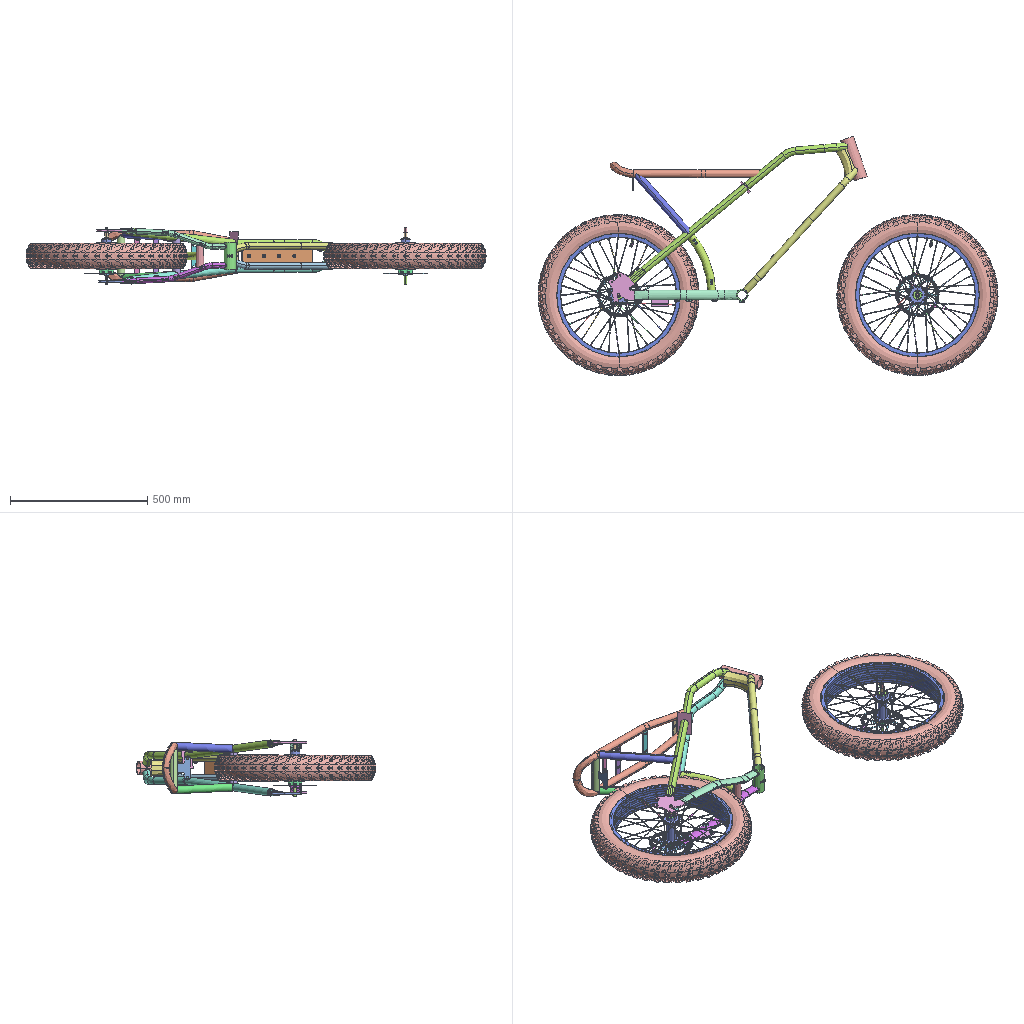Assembly | STEP file | 125 different items | 225 placed | box 1675 x 872 x 210 mm
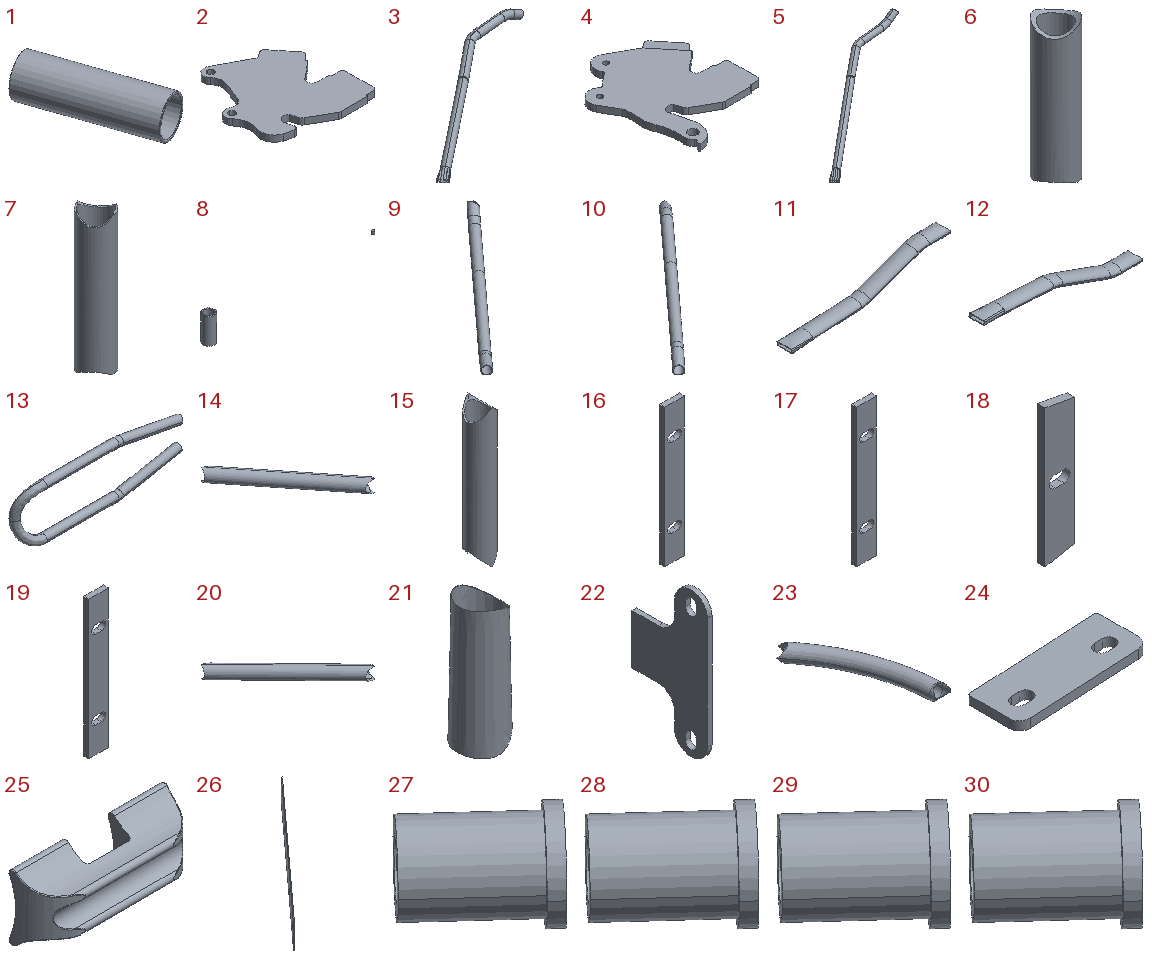Parts list (item | name | quantity | parent item | size | volume):
1 | PRT0001_68_1 | x1 | in PRT0001_68_ASM | 97.464 x 162.507 x 50 mm | 68590 mm3
2 | PRT0001_68_2 | x1 | in PRT0001_68_ASM | 96.462 x 102.711 x 6 mm | 37428 mm3
3 | PRT0001_68_3 | x1 | in PRT0001_68_ASM | 800.156 x 514.114 x 98.789 mm | 118663 mm3
4 | PRT0001_68_4 | x1 | in PRT0001_68_ASM | 102.996 x 124.109 x 6.875 mm | 43677 mm3
5 | PRT0001_68_5 | x1 | in PRT0001_68_ASM | 800.156 x 514.114 x 98.789 mm | 118661 mm3
6 | PRT0001_68_6 | x1 | in PRT0001_68_ASM | 19.001 x 19.001 x 71.436 mm | 7755 mm3
7 | PRT0001_68_7 | x1 | in PRT0001_68_ASM | 28.01 x 28.01 x 125 mm | 14806 mm3
8 | PRT0001_68_8 | x1 | in PRT0001_68_ASM | 664.5 x 43 x 100 mm | 56748 mm3
9 | PRT0001_68_9 | x1 | in PRT0001_68_ASM | 418.507 x 458.308 x 40.27 mm | 65357 mm3
10 | PRT0001_68_10 | x1 | in PRT0001_68_ASM | 418.507 x 458.308 x 40.27 mm | 65357 mm3
11 | PRT0001_68_11 | x1 | in PRT0001_68_ASM | 380.555 x 36.2 x 75.962 mm | 44196 mm3
12 | PRT0001_68_12 | x1 | in PRT0001_68_ASM | 380.555 x 36.2 x 75.962 mm | 44196 mm3
13 | PRT0001_68_13 | x1 | in PRT0001_68_ASM | 553.703 x 55.695 x 188 mm | 147514 mm3
14 | PRT0001_68_15 | x1 | in PRT0001_68_ASM | 199.467 x 218.482 x 38.316 mm | 33314 mm3
15 | PRT0001_68_16 | x1 | in PRT0001_68_ASM | 28 x 28 x 159.999 mm | 17361 mm3
16 | PRT0001_68_17 | x1 | in PRT0001_68_ASM | 20 x 5 x 138.552 mm | 12873 mm3
17 | PRT0001_68_18 | x1 | in PRT0001_68_ASM | 20 x 5 x 138.552 mm | 12873 mm3
18 | PRT0001_68_19 | x1 | in PRT0001_68_ASM | 20 x 5 x 93.385 mm | 8469 mm3
19 | PRT0001_68_20 | x1 | in PRT0001_68_ASM | 20 x 5.003 x 138.552 mm | 12879 mm3
20 | PRT0001_68_21 | x1 | in PRT0001_68_ASM | 199.467 x 218.482 x 38.316 mm | 33312 mm3
21 | PRT0001_68_22 | x1 | in PRT0001_68_ASM | 29.224 x 29.394 x 81.102 mm | 9192 mm3
22 | PRT0001_68_23 | x1 | in PRT0001_68_ASM | 2.865 x 46.012 x 88.1 mm | 6874 mm3
23 | PRT0001_68_24 | x1 | in PRT0001_68_ASM | 109.297 x 231.955 x 28 mm | 28262 mm3
24 | PRT0001_68_25 | x1 | in PRT0001_68_ASM | 62.055 x 25 x 7.544 mm | 6128 mm3
25 | PRT0001_68_27 | x11 | in PRT0001_68_ASM, PRT0001_ASM | 19.974 x 5.821 x 8.525 mm | 410.28 mm3
26 | PRT0001_68_28 | x1 | in PRT0001_68_ASM | 256.776 x 282.202 x 48 mm | 26740 mm3
27 | PRT0001_68_29 | x1 | in PRT0001_68_ASM | 20.651 x 20.315 x 13 mm | 1037 mm3
28 | PRT0001_68_30 | x1 | in PRT0001_68_ASM | 20.651 x 20.315 x 13 mm | 1037 mm3
29 | PRT0001_68_31 | x1 | in PRT0001_68_ASM | 20.651 x 20.315 x 13 mm | 1037 mm3
30 | PRT0001_68_32 | x1 | in PRT0001_68_ASM | 20.651 x 20.315 x 13 mm | 1037 mm3
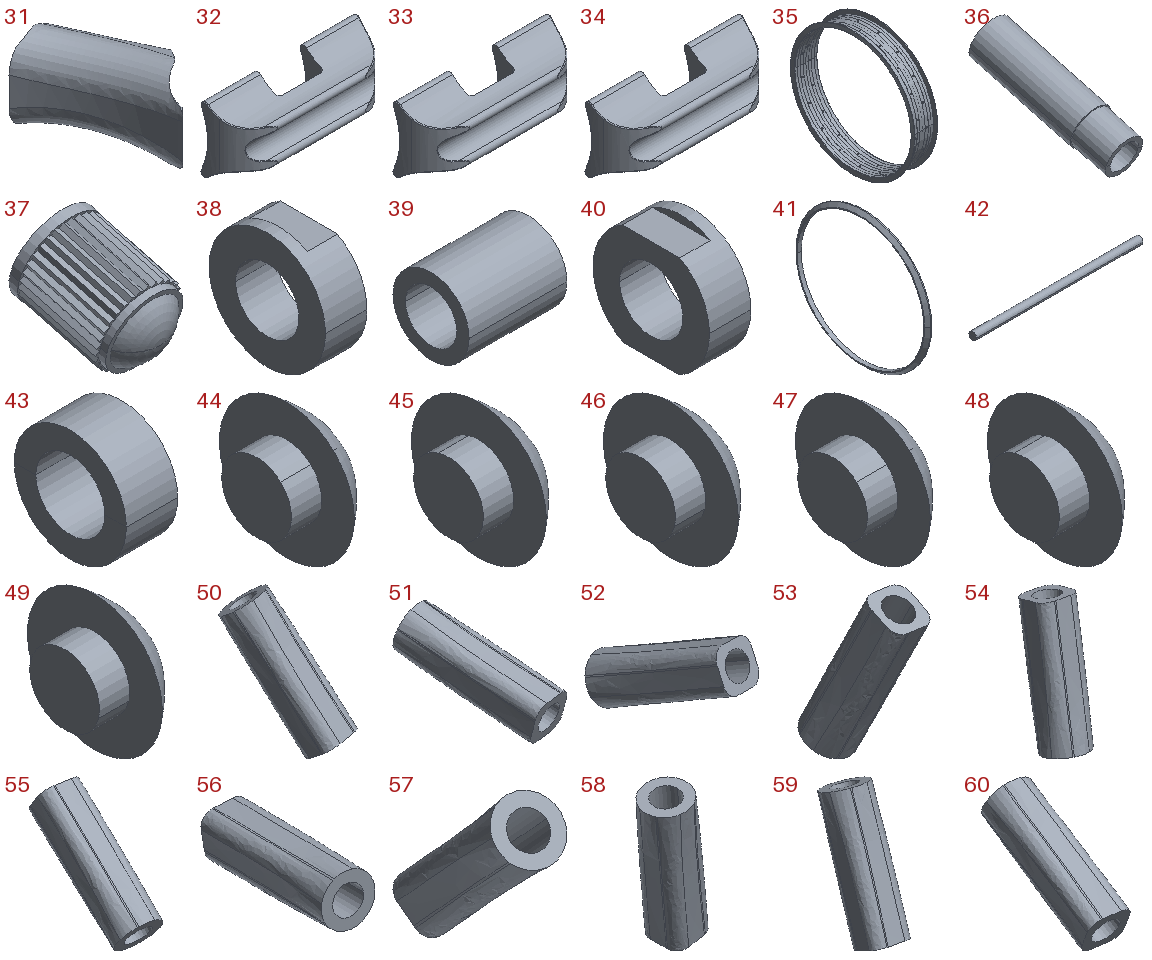31 | PRT0001_68_33 | x1 | in PRT0001_68_ASM | 68.382 x 110.355 x 61.109 mm | 20597 mm3
32 | PRT0003 | x1 | in PRT0001_ASM | 19.974 x 5.821 x 8.525 mm | 410.28 mm3
33 | PRT0004 | x1 | in PRT0001_ASM | 19.974 x 5.821 x 8.525 mm | 410.28 mm3
34 | PRT0005 | x1 | in PRT0001_ASM | 19.974 x 5.821 x 8.525 mm | 410.28 mm3
35 | BREP_1 | x2 | in FATBIKE20X4INCHFRONTWHEELAVID16_ASM | 83.255 x 451.856 x 451.856 mm | 216324 mm3
36 | BREP_2 | x2 | in FATBIKE20X4INCHFRONTWHEELAVID16_ASM | 8 x 29.756 x 14.922 mm | 672.27 mm3
37 | BREP_3 | x2 | in FATBIKE20X4INCHFRONTWHEELAVID16_ASM | 10.16 x 14.692 x 12.577 mm | 395.376 mm3
38 | BREP_4 | x2 | in FATBIKE20X4INCHFRONTWHEELAVID16_ASM | 6.16 x 17.28 x 17.28 mm | 959.564 mm3
39 | BREP_5 | x2 | in FATBIKE20X4INCHFRONTWHEELAVID16_ASM | 18 x 14 x 14 mm | 1522 mm3
40 | BREP_6 | x2 | in FATBIKE20X4INCHFRONTWHEELAVID16_ASM | 6.16 x 17.28 x 17.28 mm | 959.564 mm3
41 | BREP_7 | x2 | in FATBIKE20X4INCHFRONTWHEELAVID16_ASM | 1 x 33.32 x 33.32 mm | 72.205 mm3
42 | BREP_8 | x2 | in FATBIKE20X4INCHFRONTWHEELAVID16_ASM | 210 x 9.4 x 9.4 mm | 14574 mm3
43 | BREP_9 | x2 | in FATBIKE20X4INCHFRONTWHEELAVID16_ASM | 7 x 15.25 x 15.25 mm | 792.795 mm3
44 | OBJECT_38-2315 | x2 | in FATBIKE20X4INCHFRONTWHEELAVID16_ASM | 3.344 x 7.727 x 7.727 mm | 53.316 mm3
45 | OBJECT_38-2316 | x2 | in FATBIKE20X4INCHFRONTWHEELAVID16_ASM | 3.344 x 7.727 x 7.727 mm | 53.316 mm3
46 | OBJECT_38-2317 | x2 | in FATBIKE20X4INCHFRONTWHEELAVID16_ASM | 3.344 x 7.727 x 7.727 mm | 53.316 mm3
47 | OBJECT_38-2318 | x2 | in FATBIKE20X4INCHFRONTWHEELAVID16_ASM | 3.344 x 7.727 x 7.727 mm | 53.316 mm3
48 | OBJECT_38-2319 | x2 | in FATBIKE20X4INCHFRONTWHEELAVID16_ASM | 3.344 x 7.727 x 7.727 mm | 53.316 mm3
49 | OBJECT_38-2320 | x2 | in FATBIKE20X4INCHFRONTWHEELAVID16_ASM | 3.344 x 7.727 x 7.727 mm | 53.316 mm3
50 | BREP_16 | x2 | in FATBIKE20X4INCHFRONTWHEELAVID16_ASM | 5.376 x 10.304 x 11.842 mm | 92.736 mm3
51 | BREP_17 | x2 | in FATBIKE20X4INCHFRONTWHEELAVID16_ASM | 5.376 x 12.643 x 6.336 mm | 92.736 mm3
52 | BREP_18 | x2 | in FATBIKE20X4INCHFRONTWHEELAVID16_ASM | 5.376 x 12.425 x 8.884 mm | 92.736 mm3
53 | BREP_19 | x2 | in FATBIKE20X4INCHFRONTWHEELAVID16_ASM | 5.376 x 8.093 x 12.59 mm | 92.736 mm3
54 | BREP_20 | x2 | in FATBIKE20X4INCHFRONTWHEELAVID16_ASM | 5.376 x 7.197 x 12.647 mm | 92.736 mm3
55 | BREP_21 | x2 | in FATBIKE20X4INCHFRONTWHEELAVID16_ASM | 5.376 x 12.182 x 9.645 mm | 92.736 mm3
56 | BREP_22 | x2 | in FATBIKE20X4INCHFRONTWHEELAVID16_ASM | 5.376 x 12.545 x 5.293 mm | 92.736 mm3
57 | BREP_23 | x2 | in FATBIKE20X4INCHFRONTWHEELAVID16_ASM | 5.376 x 10.907 x 11.414 mm | 92.736 mm3
58 | BREP_24 | x2 | in FATBIKE20X4INCHFRONTWHEELAVID16_ASM | 5.376 x 4.387 x 12.44 mm | 92.736 mm3
59 | BREP_25 | x2 | in FATBIKE20X4INCHFRONTWHEELAVID16_ASM | 5.376 x 8.884 x 12.425 mm | 92.736 mm3
60 | BREP_26 | x2 | in FATBIKE20X4INCHFRONTWHEELAVID16_ASM | 5.376 x 12.59 x 8.093 mm | 92.736 mm3
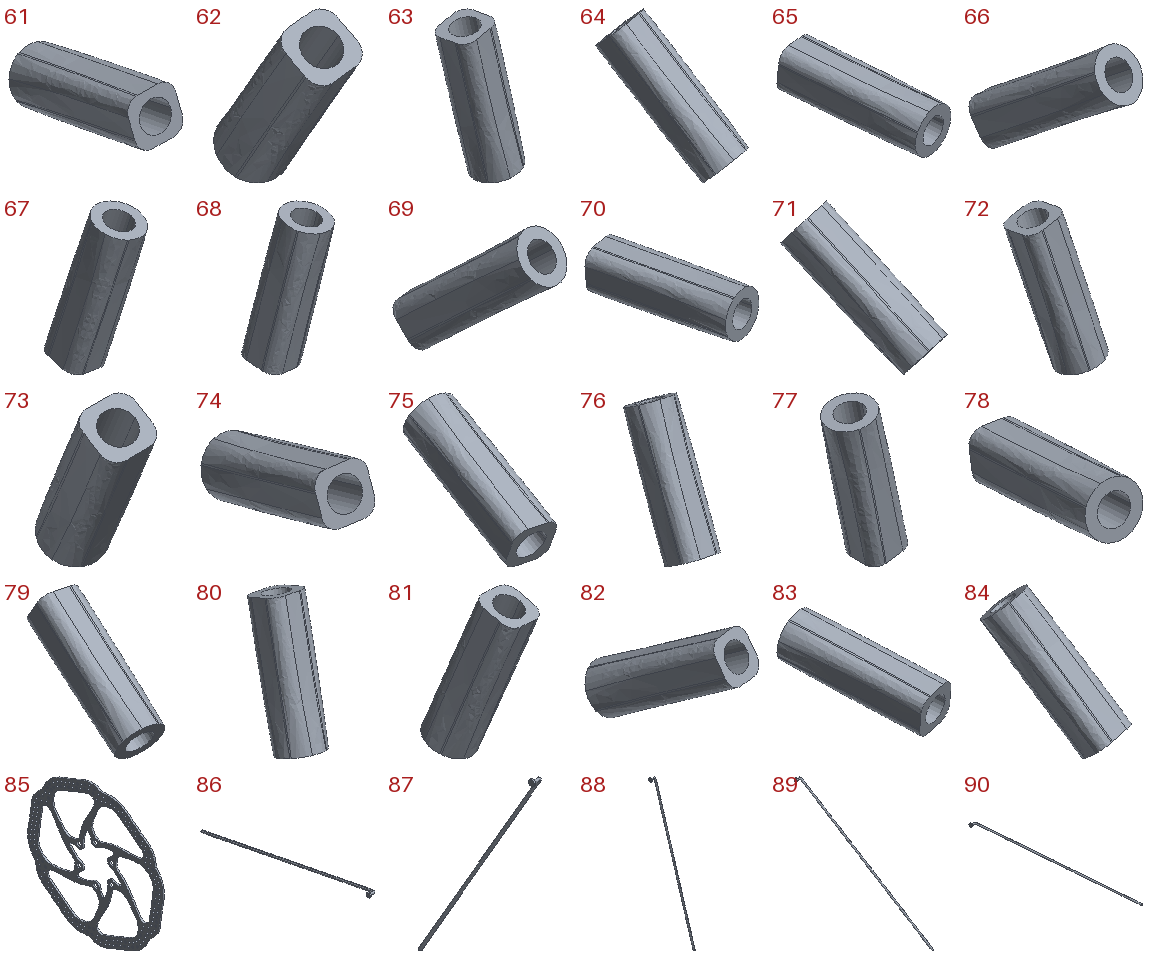61 | BREP_27 | x2 | in FATBIKE20X4INCHFRONTWHEELAVID16_ASM | 5.376 x 12.647 x 7.197 mm | 92.736 mm3
62 | BREP_28 | x2 | in FATBIKE20X4INCHFRONTWHEELAVID16_ASM | 5.376 x 9.645 x 12.182 mm | 92.736 mm3
63 | BREP_29 | x2 | in FATBIKE20X4INCHFRONTWHEELAVID16_ASM | 5.376 x 5.293 x 12.545 mm | 92.736 mm3
64 | BREP_30 | x2 | in FATBIKE20X4INCHFRONTWHEELAVID16_ASM | 5.376 x 11.414 x 10.907 mm | 92.736 mm3
65 | BREP_31 | x2 | in FATBIKE20X4INCHFRONTWHEELAVID16_ASM | 5.376 x 12.44 x 4.387 mm | 92.736 mm3
66 | BREP_32 | x2 | in FATBIKE20X4INCHFRONTWHEELAVID16_ASM | 5.376 x 11.842 x 10.304 mm | 92.736 mm3
67 | BREP_33 | x2 | in FATBIKE20X4INCHFRONTWHEELAVID16_ASM | 5.376 x 6.336 x 12.643 mm | 92.736 mm3
68 | BREP_34 | x2 | in FATBIKE20X4INCHFRONTWHEELAVID16_ASM | 5.786 x 5.283 x 12.591 mm | 92.736 mm3
69 | BREP_35 | x2 | in FATBIKE20X4INCHFRONTWHEELAVID16_ASM | 5.786 x 11.394 x 10.896 mm | 92.736 mm3
70 | BREP_36 | x2 | in FATBIKE20X4INCHFRONTWHEELAVID16_ASM | 5.786 x 12.504 x 4.377 mm | 92.736 mm3
71 | BREP_37 | x2 | in FATBIKE20X4INCHFRONTWHEELAVID16_ASM | 5.786 x 11.833 x 10.283 mm | 92.736 mm3
72 | BREP_38 | x2 | in FATBIKE20X4INCHFRONTWHEELAVID16_ASM | 5.786 x 6.31 x 12.663 mm | 92.736 mm3
73 | BREP_39 | x2 | in FATBIKE20X4INCHFRONTWHEELAVID16_ASM | 5.786 x 8.865 x 12.421 mm | 92.736 mm3
74 | BREP_40 | x2 | in FATBIKE20X4INCHFRONTWHEELAVID16_ASM | 5.786 x 12.586 x 8.086 mm | 92.736 mm3
75 | BREP_41 | x2 | in FATBIKE20X4INCHFRONTWHEELAVID16_ASM | 5.786 x 12.658 x 7.181 mm | 92.736 mm3
76 | BREP_42 | x2 | in FATBIKE20X4INCHFRONTWHEELAVID16_ASM | 5.786 x 9.635 x 12.167 mm | 92.736 mm3
77 | BREP_43 | x2 | in FATBIKE20X4INCHFRONTWHEELAVID16_ASM | 5.786 x 4.377 x 12.504 mm | 92.736 mm3
78 | BREP_44 | x2 | in FATBIKE20X4INCHFRONTWHEELAVID16_ASM | 5.786 x 12.663 x 6.31 mm | 92.736 mm3
79 | BREP_45 | x2 | in FATBIKE20X4INCHFRONTWHEELAVID16_ASM | 5.786 x 12.421 x 8.865 mm | 92.736 mm3
80 | BREP_46 | x2 | in FATBIKE20X4INCHFRONTWHEELAVID16_ASM | 5.786 x 8.086 x 12.586 mm | 92.736 mm3
81 | BREP_47 | x2 | in FATBIKE20X4INCHFRONTWHEELAVID16_ASM | 5.786 x 7.181 x 12.658 mm | 92.736 mm3
82 | BREP_48 | x2 | in FATBIKE20X4INCHFRONTWHEELAVID16_ASM | 5.786 x 12.167 x 9.635 mm | 92.736 mm3
83 | BREP_49 | x2 | in FATBIKE20X4INCHFRONTWHEELAVID16_ASM | 5.786 x 12.591 x 5.283 mm | 92.736 mm3
84 | BREP_50 | x2 | in FATBIKE20X4INCHFRONTWHEELAVID16_ASM | 5.786 x 10.896 x 11.394 mm | 92.736 mm3
85 | BREP_51 | x2 | in FATBIKE20X4INCHFRONTWHEELAVID16_ASM | 1.8 x 158.335 x 159.5 mm | 12555 mm3
86 | BREP_52 | x2 | in FATBIKE20X4INCHFRONTWHEELAVID16_ASM | 33.776 x 193.437 x 62.153 mm | 645.284 mm3
87 | BREP_53 | x2 | in FATBIKE20X4INCHFRONTWHEELAVID16_ASM | 33.776 x 111.192 x 170.747 mm | 645.284 mm3
88 | BREP_54 | x2 | in FATBIKE20X4INCHFRONTWHEELAVID16_ASM | 33.776 x 28.103 x 200.673 mm | 645.284 mm3
89 | BREP_55 | x2 | in FATBIKE20X4INCHFRONTWHEELAVID16_ASM | 33.776 x 149.51 x 138.649 mm | 645.284 mm3
90 | BREP_56 | x2 | in FATBIKE20X4INCHFRONTWHEELAVID16_ASM | 33.776 x 201.979 x 12.73 mm | 645.284 mm3
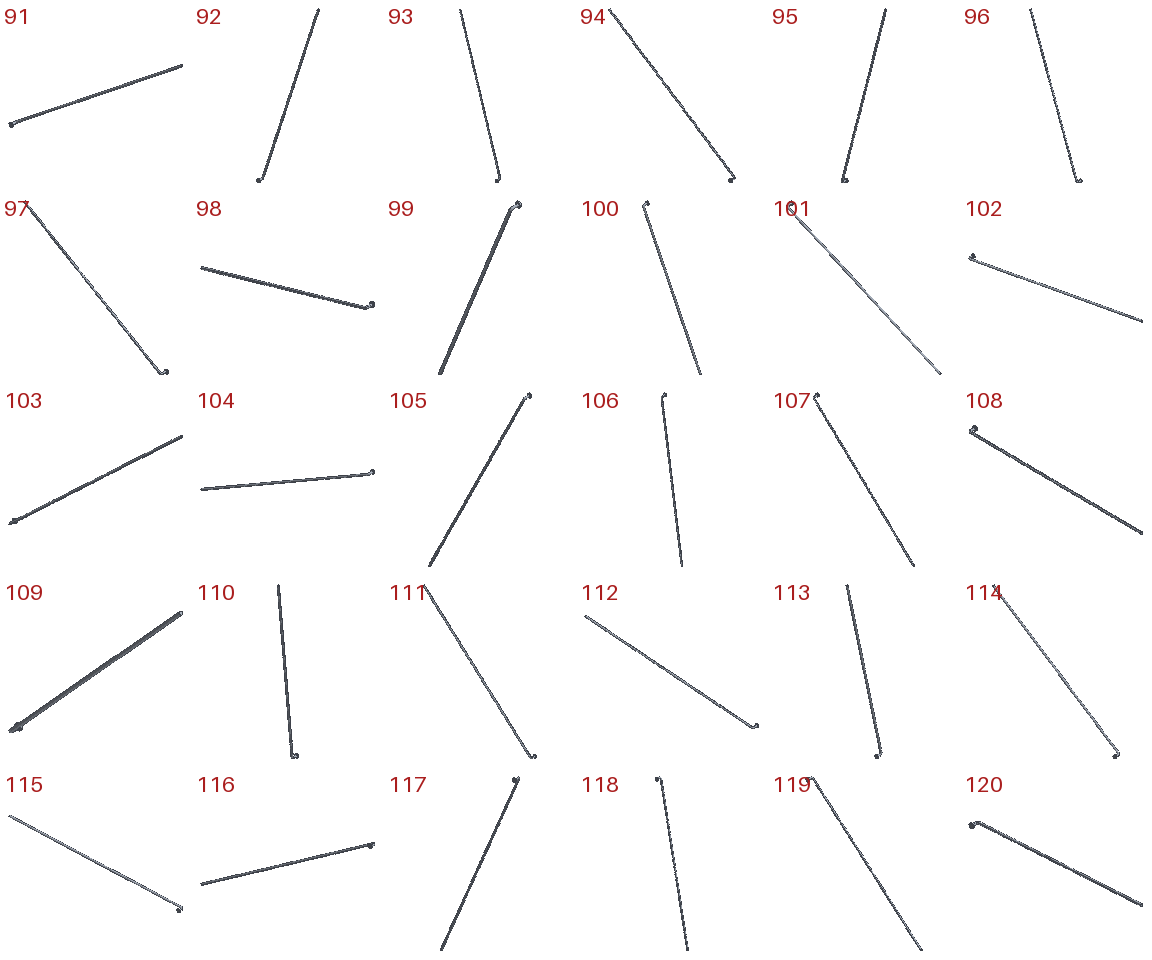91 | BREP_57 | x2 | in FATBIKE20X4INCHFRONTWHEELAVID16_ASM | 33.776 x 161.956 x 123.792 mm | 645.284 mm3
92 | BREP_58 | x2 | in FATBIKE20X4INCHFRONTWHEELAVID16_ASM | 33.776 x 47.261 x 197.368 mm | 645.284 mm3
93 | BREP_59 | x2 | in FATBIKE20X4INCHFRONTWHEELAVID16_ASM | 33.776 x 94.376 x 180.404 mm | 645.284 mm3
94 | BREP_60 | x2 | in FATBIKE20X4INCHFRONTWHEELAVID16_ASM | 33.776 x 186.861 x 80.417 mm | 645.284 mm3
95 | BREP_61 | x2 | in FATBIKE20X4INCHFRONTWHEELAVID16_ASM | 35.925 x 28.108 x 200.702 mm | 653.861 mm3
96 | BREP_62 | x2 | in FATBIKE20X4INCHFRONTWHEELAVID16_ASM | 35.925 x 111.196 x 170.756 mm | 653.86 mm3
97 | BREP_63 | x2 | in FATBIKE20X4INCHFRONTWHEELAVID16_ASM | 35.925 x 193.453 x 62.159 mm | 653.86 mm3
98 | BREP_64 | x2 | in FATBIKE20X4INCHFRONTWHEELAVID16_ASM | 35.925 x 186.872 x 80.422 mm | 653.861 mm3
99 | BREP_65 | x2 | in FATBIKE20X4INCHFRONTWHEELAVID16_ASM | 35.925 x 94.382 x 180.414 mm | 653.861 mm3
100 | BREP_66 | x2 | in FATBIKE20X4INCHFRONTWHEELAVID16_ASM | 35.925 x 47.266 x 197.386 mm | 653.861 mm3
101 | BREP_67 | x2 | in FATBIKE20X4INCHFRONTWHEELAVID16_ASM | 35.925 x 161.962 x 123.799 mm | 653.86 mm3
102 | BREP_68 | x2 | in FATBIKE20X4INCHFRONTWHEELAVID16_ASM | 35.925 x 202.012 x 12.735 mm | 653.861 mm3
103 | BREP_69 | x2 | in FATBIKE20X4INCHFRONTWHEELAVID16_ASM | 35.925 x 149.517 x 138.654 mm | 653.861 mm3
104 | BREP_70 | x2 | in FATBIKE20X4INCHFRONTWHEELAVID16_ASM | 33.776 x 180.404 x 94.376 mm | 676.26 mm3
105 | BREP_71 | x2 | in FATBIKE20X4INCHFRONTWHEELAVID16_ASM | 33.776 x 80.417 x 186.861 mm | 676.26 mm3
106 | BREP_72 | x2 | in FATBIKE20X4INCHFRONTWHEELAVID16_ASM | 33.776 x 62.153 x 193.437 mm | 676.26 mm3
107 | BREP_73 | x2 | in FATBIKE20X4INCHFRONTWHEELAVID16_ASM | 33.776 x 170.747 x 111.192 mm | 676.26 mm3
108 | BREP_74 | x2 | in FATBIKE20X4INCHFRONTWHEELAVID16_ASM | 33.776 x 200.673 x 28.103 mm | 676.26 mm3
109 | BREP_75 | x2 | in FATBIKE20X4INCHFRONTWHEELAVID16_ASM | 33.776 x 138.649 x 149.51 mm | 676.26 mm3
110 | BREP_76 | x2 | in FATBIKE20X4INCHFRONTWHEELAVID16_ASM | 33.776 x 12.73 x 201.979 mm | 676.26 mm3
111 | BREP_77 | x2 | in FATBIKE20X4INCHFRONTWHEELAVID16_ASM | 33.776 x 123.792 x 161.956 mm | 676.26 mm3
112 | BREP_78 | x2 | in FATBIKE20X4INCHFRONTWHEELAVID16_ASM | 33.776 x 197.368 x 47.261 mm | 676.26 mm3
113 | BREP_79 | x2 | in FATBIKE20X4INCHFRONTWHEELAVID16_ASM | 35.925 x 12.735 x 202.012 mm | 668.221 mm3
114 | BREP_80 | x2 | in FATBIKE20X4INCHFRONTWHEELAVID16_ASM | 35.925 x 138.654 x 149.517 mm | 668.221 mm3
115 | BREP_81 | x2 | in FATBIKE20X4INCHFRONTWHEELAVID16_ASM | 35.925 x 200.702 x 28.108 mm | 668.221 mm3
116 | BREP_82 | x2 | in FATBIKE20X4INCHFRONTWHEELAVID16_ASM | 35.925 x 170.756 x 111.196 mm | 668.221 mm3
117 | BREP_83 | x2 | in FATBIKE20X4INCHFRONTWHEELAVID16_ASM | 35.925 x 62.159 x 193.453 mm | 668.221 mm3
118 | BREP_84 | x2 | in FATBIKE20X4INCHFRONTWHEELAVID16_ASM | 35.925 x 80.422 x 186.872 mm | 668.221 mm3
119 | BREP_85 | x2 | in FATBIKE20X4INCHFRONTWHEELAVID16_ASM | 35.925 x 180.414 x 94.382 mm | 668.221 mm3
120 | BREP_86 | x2 | in FATBIKE20X4INCHFRONTWHEELAVID16_ASM | 35.925 x 197.386 x 47.266 mm | 668.221 mm3
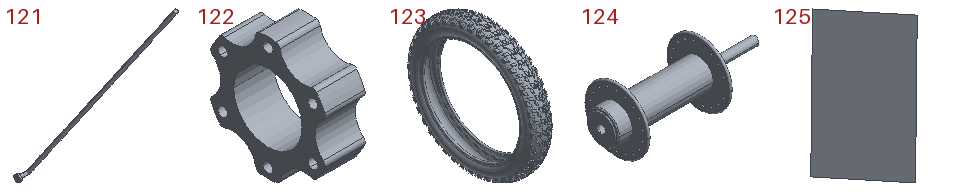121 | BREP_87 | x2 | in FATBIKE20X4INCHFRONTWHEELAVID16_ASM | 35.925 x 123.799 x 161.962 mm | 668.221 mm3
122 | BREP_88 | x2 | in FATBIKE20X4INCHFRONTWHEELAVID16_ASM | 17 x 48.379 x 52 mm | 16406 mm3
123 | BREP_89 | x2 | in FATBIKE20X4INCHFRONTWHEELAVID16_ASM | 94.52 x 587.169 x 587.169 mm | 1952183 mm3
124 | COMPOUND | x2 | in FATBIKE20X4INCHFRONTWHEELAVID16_ASM | - | -
125 | PRT0001_68_3_ASM | x1 | in PRT0001_ASM | - | -
Placements (level | parent | child | x y z in mm | rotation matrix by rows), first 212 of 228 lines:
1 | PRT0001_ASM | PRT0001_68_ASM | 0.0 0.0 0.0 | 1 0 0 0 1 0 0 0 1
2 | PRT0001_68_ASM | PRT0001_68_1 | 0.0 0.0 0.0 | 1 0 0 0 1 0 0 0 1
2 | PRT0001_68_ASM | PRT0001_68_2 | 0.0 0.0 0.0 | 1 0 0 0 1 0 0 0 1
2 | PRT0001_68_ASM | PRT0001_68_3 | 0.0 0.0 0.0 | 1 0 0 0 1 0 0 0 1
2 | PRT0001_68_ASM | PRT0001_68_4 | 0.0 0.0 0.0 | 1 0 0 0 1 0 0 0 1
2 | PRT0001_68_ASM | PRT0001_68_5 | 0.0 0.0 0.0 | 1 0 0 0 1 0 0 0 1
2 | PRT0001_68_ASM | PRT0001_68_6 | 0.0 0.0 0.0 | 1 0 0 0 1 0 0 0 1
2 | PRT0001_68_ASM | PRT0001_68_7 | 0.0 0.0 0.0 | 1 0 0 0 1 0 0 0 1
2 | PRT0001_68_ASM | PRT0001_68_8 | 0.0 0.0 0.0 | 1 0 0 0 1 0 0 0 1
2 | PRT0001_68_ASM | PRT0001_68_9 | 0.0 0.0 0.0 | 1 0 0 0 1 0 0 0 1
2 | PRT0001_68_ASM | PRT0001_68_10 | 0.0 0.0 0.0 | 1 0 0 0 1 0 0 0 1
2 | PRT0001_68_ASM | PRT0001_68_11 | 0.0 0.0 0.0 | 1 0 0 0 1 0 0 0 1
2 | PRT0001_68_ASM | PRT0001_68_12 | 0.0 0.0 0.0 | 1 0 0 0 1 0 0 0 1
2 | PRT0001_68_ASM | PRT0001_68_13 | 0.0 0.0 0.0 | 1 0 0 0 1 0 0 0 1
2 | PRT0001_68_ASM | PRT0001_68_15 | 0.0 0.0 0.0 | 1 0 0 0 1 0 0 0 1
2 | PRT0001_68_ASM | PRT0001_68_16 | 0.0 0.0 0.0 | 1 0 0 0 1 0 0 0 1
2 | PRT0001_68_ASM | PRT0001_68_17 | 0.0 0.0 0.0 | 1 0 0 0 1 0 0 0 1
2 | PRT0001_68_ASM | PRT0001_68_18 | 0.0 0.0 0.0 | 1 0 0 0 1 0 0 0 1
2 | PRT0001_68_ASM | PRT0001_68_19 | 0.0 0.0 0.0 | 1 0 0 0 1 0 0 0 1
2 | PRT0001_68_ASM | PRT0001_68_20 | 0.0 0.0 0.0 | 1 0 0 0 1 0 0 0 1
2 | PRT0001_68_ASM | PRT0001_68_21 | 0.0 0.0 0.0 | 1 0 0 0 1 0 0 0 1
2 | PRT0001_68_ASM | PRT0001_68_22 | 0.0 0.0 0.0 | 1 0 0 0 1 0 0 0 1
2 | PRT0001_68_ASM | PRT0001_68_23 | 0.0 0.0 0.0 | 1 0 0 0 1 0 0 0 1
2 | PRT0001_68_ASM | PRT0001_68_24 | 0.0 0.0 0.0 | 1 0 0 0 1 0 0 0 1
2 | PRT0001_68_ASM | PRT0001_68_25 | 0.0 0.0 0.0 | 1 0 0 0 1 0 0 0 1
2 | PRT0001_68_ASM | PRT0001_68_27 | 0.0 0.6126 0.0 | 1 0 0 0 1 0 0 0 1
2 | PRT0001_68_ASM | PRT0001_68_28 | 0.0 0.0 0.0 | 1 0 0 0 1 0 0 0 1
2 | PRT0001_68_ASM | PRT0001_68_29 | 0.0 0.0 0.0 | 1 0 0 0 1 0 0 0 1
2 | PRT0001_68_ASM | PRT0001_68_30 | 0.0 0.0 0.0 | 1 0 0 0 1 0 0 0 1
2 | PRT0001_68_ASM | PRT0001_68_31 | 0.0 0.0 0.0 | 1 0 0 0 1 0 0 0 1
2 | PRT0001_68_ASM | PRT0001_68_32 | 0.0 0.0 0.0 | 1 0 0 0 1 0 0 0 1
2 | PRT0001_68_ASM | PRT0001_68_33 | 0.0 0.0 0.0 | 1 0 0 0 1 0 0 0 1
1 | PRT0001_ASM | PRT0001_68_27 | 759.008 -0.9936 -720.263 | 0.6727 0.1695 0.7202 0.7399 -0.1541 -0.6548 0 0.9734 -0.2291
1 | PRT0001_ASM | PRT0001_68_27 | -8.194 4.929 600.004 | 0.9458 0 0.3249 0 1 0 -0.3249 0 0.9458
1 | PRT0001_ASM | PRT0001_68_27 | -101.99 4.929 633.188 | 0.9458 0 0.3249 0 1 0 -0.3249 0 0.9458
1 | PRT0001_ASM | PRT0001_68_27 | -235.333 4.929 185.767 | 0.9983 0 0.05791 0 1 0 -0.05791 0 0.9983
1 | PRT0001_ASM | PRT0001_68_27 | -344.15 -56.9 -174.443 | 0.9984 -0.03645 -0.04359 0.03601 0.9993 -0.01103 0.04396 0.009441 0.999
1 | PRT0001_ASM | PRT0003 | -8.194 4.929 -600.004 | 0.9458 0 -0.3249 0 1 0 0.3249 0 0.9458
1 | PRT0001_ASM | PRT0004 | -101.99 4.929 -633.188 | 0.9458 0 -0.3249 0 1 0 0.3249 0 0.9458
1 | PRT0001_ASM | PRT0005 | -235.333 4.929 -185.767 | 0.9983 0 -0.05791 0 1 0 0.05791 0 0.9983
1 | PRT0001_ASM | PRT0001_68_27 | 241.304 2084.491 549.844 | 0.6887 0.03142 0.7244 -0.7207 -0.0795 0.6886 0.07922 -0.9963 -0.0321
1 | PRT0001_ASM | PRT0001_68_27 | 1684.219 2560.128 747.789 | 0.05271 -0.2251 0.9729 -0.9986 -0.01795 0.04995 0.006222 -0.9742 -0.2257
1 | PRT0001_ASM | PRT0001_68_27 | 745.623 2477.22 817.741 | 0.5497 -0.1886 0.8138 -0.8347 -0.08612 0.5439 -0.03247 -0.9783 -0.2047
1 | PRT0001_ASM | PRT0001_68_27 | 401.651 2363.862 -699.778 | 0.6347 0.00596 -0.7727 -0.7727 -0.000694 -0.6347 -0.004319 1 0.004165
1 | PRT0001_ASM | PRT0001_68_27 | 237.023 2452.022 -692.669 | 0.659 0.01631 -0.752 -0.7521 0.007809 -0.659 -0.004876 0.9998 0.01741
1 | PRT0001_ASM | FATBIKE20X4INCHFRONTWHEELAVID16_ASM | 2352.479 786.478 0.0 | 0 0 1 0 1 0 -1 0 0
2 | FATBIKE20X4INCHFRONTWHEELAVID16_ASM | BREP_1 | 0.0 0.0 0.0 | 1 0 0 0 1 0 0 0 1
2 | FATBIKE20X4INCHFRONTWHEELAVID16_ASM | BREP_2 | 0.0 0.0 0.0 | 1 0 0 0 1 0 0 0 1
2 | FATBIKE20X4INCHFRONTWHEELAVID16_ASM | BREP_3 | 0.0 0.0 0.0 | 1 0 0 0 1 0 0 0 1
2 | FATBIKE20X4INCHFRONTWHEELAVID16_ASM | BREP_4 | 0.0 0.0 0.0 | 1 0 0 0 1 0 0 0 1
2 | FATBIKE20X4INCHFRONTWHEELAVID16_ASM | BREP_5 | 0.0 0.0 0.0 | 1 0 0 0 1 0 0 0 1
2 | FATBIKE20X4INCHFRONTWHEELAVID16_ASM | BREP_6 | 0.0 0.0 0.0 | 1 0 0 0 1 0 0 0 1
2 | FATBIKE20X4INCHFRONTWHEELAVID16_ASM | BREP_7 | 0.0 0.0 0.0 | 1 0 0 0 1 0 0 0 1
2 | FATBIKE20X4INCHFRONTWHEELAVID16_ASM | BREP_8 | 0.0 0.0 0.0 | 1 0 0 0 1 0 0 0 1
2 | FATBIKE20X4INCHFRONTWHEELAVID16_ASM | BREP_9 | 0.0 0.0 0.0 | 1 0 0 0 1 0 0 0 1
2 | FATBIKE20X4INCHFRONTWHEELAVID16_ASM | OBJECT_38-2315 | 0.0 0.0 0.0 | 1 0 0 0 1 0 0 0 1
2 | FATBIKE20X4INCHFRONTWHEELAVID16_ASM | OBJECT_38-2316 | 0.0 0.0 0.0 | 1 0 0 0 1 0 0 0 1
2 | FATBIKE20X4INCHFRONTWHEELAVID16_ASM | OBJECT_38-2317 | 0.0 0.0 0.0 | 1 0 0 0 1 0 0 0 1
2 | FATBIKE20X4INCHFRONTWHEELAVID16_ASM | OBJECT_38-2318 | 0.0 0.0 0.0 | 1 0 0 0 1 0 0 0 1
2 | FATBIKE20X4INCHFRONTWHEELAVID16_ASM | OBJECT_38-2319 | 0.0 0.0 0.0 | 1 0 0 0 1 0 0 0 1
2 | FATBIKE20X4INCHFRONTWHEELAVID16_ASM | OBJECT_38-2320 | 0.0 0.0 0.0 | 1 0 0 0 1 0 0 0 1
2 | FATBIKE20X4INCHFRONTWHEELAVID16_ASM | BREP_16 | 0.0 0.0 0.0 | 1 0 0 0 1 0 0 0 1
2 | FATBIKE20X4INCHFRONTWHEELAVID16_ASM | BREP_17 | 0.0 0.0 0.0 | 1 0 0 0 1 0 0 0 1
2 | FATBIKE20X4INCHFRONTWHEELAVID16_ASM | BREP_18 | 0.0 0.0 0.0 | 1 0 0 0 1 0 0 0 1
2 | FATBIKE20X4INCHFRONTWHEELAVID16_ASM | BREP_19 | 0.0 0.0 0.0 | 1 0 0 0 1 0 0 0 1
2 | FATBIKE20X4INCHFRONTWHEELAVID16_ASM | BREP_20 | 0.0 0.0 0.0 | 1 0 0 0 1 0 0 0 1
2 | FATBIKE20X4INCHFRONTWHEELAVID16_ASM | BREP_21 | 0.0 0.0 0.0 | 1 0 0 0 1 0 0 0 1
2 | FATBIKE20X4INCHFRONTWHEELAVID16_ASM | BREP_22 | 0.0 0.0 0.0 | 1 0 0 0 1 0 0 0 1
2 | FATBIKE20X4INCHFRONTWHEELAVID16_ASM | BREP_23 | 0.0 0.0 0.0 | 1 0 0 0 1 0 0 0 1
2 | FATBIKE20X4INCHFRONTWHEELAVID16_ASM | BREP_24 | 0.0 0.0 0.0 | 1 0 0 0 1 0 0 0 1
2 | FATBIKE20X4INCHFRONTWHEELAVID16_ASM | BREP_25 | 0.0 0.0 0.0 | 1 0 0 0 1 0 0 0 1
2 | FATBIKE20X4INCHFRONTWHEELAVID16_ASM | BREP_26 | 0.0 0.0 0.0 | 1 0 0 0 1 0 0 0 1
2 | FATBIKE20X4INCHFRONTWHEELAVID16_ASM | BREP_27 | 0.0 0.0 0.0 | 1 0 0 0 1 0 0 0 1
2 | FATBIKE20X4INCHFRONTWHEELAVID16_ASM | BREP_28 | 0.0 0.0 0.0 | 1 0 0 0 1 0 0 0 1
2 | FATBIKE20X4INCHFRONTWHEELAVID16_ASM | BREP_29 | 0.0 0.0 0.0 | 1 0 0 0 1 0 0 0 1
2 | FATBIKE20X4INCHFRONTWHEELAVID16_ASM | BREP_30 | 0.0 0.0 0.0 | 1 0 0 0 1 0 0 0 1
2 | FATBIKE20X4INCHFRONTWHEELAVID16_ASM | BREP_31 | 0.0 0.0 0.0 | 1 0 0 0 1 0 0 0 1
2 | FATBIKE20X4INCHFRONTWHEELAVID16_ASM | BREP_32 | 0.0 0.0 0.0 | 1 0 0 0 1 0 0 0 1
2 | FATBIKE20X4INCHFRONTWHEELAVID16_ASM | BREP_33 | 0.0 0.0 0.0 | 1 0 0 0 1 0 0 0 1
2 | FATBIKE20X4INCHFRONTWHEELAVID16_ASM | BREP_34 | 0.0 0.0 0.0 | 1 0 0 0 1 0 0 0 1
2 | FATBIKE20X4INCHFRONTWHEELAVID16_ASM | BREP_35 | 0.0 0.0 0.0 | 1 0 0 0 1 0 0 0 1
2 | FATBIKE20X4INCHFRONTWHEELAVID16_ASM | BREP_36 | 0.0 0.0 0.0 | 1 0 0 0 1 0 0 0 1
2 | FATBIKE20X4INCHFRONTWHEELAVID16_ASM | BREP_37 | 0.0 0.0 0.0 | 1 0 0 0 1 0 0 0 1
2 | FATBIKE20X4INCHFRONTWHEELAVID16_ASM | BREP_38 | 0.0 0.0 0.0 | 1 0 0 0 1 0 0 0 1
2 | FATBIKE20X4INCHFRONTWHEELAVID16_ASM | BREP_39 | 0.0 0.0 0.0 | 1 0 0 0 1 0 0 0 1
2 | FATBIKE20X4INCHFRONTWHEELAVID16_ASM | BREP_40 | 0.0 0.0 0.0 | 1 0 0 0 1 0 0 0 1
2 | FATBIKE20X4INCHFRONTWHEELAVID16_ASM | BREP_41 | 0.0 0.0 0.0 | 1 0 0 0 1 0 0 0 1
2 | FATBIKE20X4INCHFRONTWHEELAVID16_ASM | BREP_42 | 0.0 0.0 0.0 | 1 0 0 0 1 0 0 0 1
2 | FATBIKE20X4INCHFRONTWHEELAVID16_ASM | BREP_43 | 0.0 0.0 0.0 | 1 0 0 0 1 0 0 0 1
2 | FATBIKE20X4INCHFRONTWHEELAVID16_ASM | BREP_44 | 0.0 0.0 0.0 | 1 0 0 0 1 0 0 0 1
2 | FATBIKE20X4INCHFRONTWHEELAVID16_ASM | BREP_45 | 0.0 0.0 0.0 | 1 0 0 0 1 0 0 0 1
2 | FATBIKE20X4INCHFRONTWHEELAVID16_ASM | BREP_46 | 0.0 0.0 0.0 | 1 0 0 0 1 0 0 0 1
2 | FATBIKE20X4INCHFRONTWHEELAVID16_ASM | BREP_47 | 0.0 0.0 0.0 | 1 0 0 0 1 0 0 0 1
2 | FATBIKE20X4INCHFRONTWHEELAVID16_ASM | BREP_48 | 0.0 0.0 0.0 | 1 0 0 0 1 0 0 0 1
2 | FATBIKE20X4INCHFRONTWHEELAVID16_ASM | BREP_49 | 0.0 0.0 0.0 | 1 0 0 0 1 0 0 0 1
2 | FATBIKE20X4INCHFRONTWHEELAVID16_ASM | BREP_50 | 0.0 0.0 0.0 | 1 0 0 0 1 0 0 0 1
2 | FATBIKE20X4INCHFRONTWHEELAVID16_ASM | BREP_51 | 0.0 0.0 0.0 | 1 0 0 0 1 0 0 0 1
2 | FATBIKE20X4INCHFRONTWHEELAVID16_ASM | BREP_52 | 0.0 0.0 0.0 | 1 0 0 0 1 0 0 0 1
2 | FATBIKE20X4INCHFRONTWHEELAVID16_ASM | BREP_53 | 0.0 0.0 0.0 | 1 0 0 0 1 0 0 0 1
2 | FATBIKE20X4INCHFRONTWHEELAVID16_ASM | BREP_54 | 0.0 0.0 0.0 | 1 0 0 0 1 0 0 0 1
2 | FATBIKE20X4INCHFRONTWHEELAVID16_ASM | BREP_55 | 0.0 0.0 0.0 | 1 0 0 0 1 0 0 0 1
2 | FATBIKE20X4INCHFRONTWHEELAVID16_ASM | BREP_56 | 0.0 0.0 0.0 | 1 0 0 0 1 0 0 0 1
2 | FATBIKE20X4INCHFRONTWHEELAVID16_ASM | BREP_57 | 0.0 0.0 0.0 | 1 0 0 0 1 0 0 0 1
2 | FATBIKE20X4INCHFRONTWHEELAVID16_ASM | BREP_58 | 0.0 0.0 0.0 | 1 0 0 0 1 0 0 0 1
2 | FATBIKE20X4INCHFRONTWHEELAVID16_ASM | BREP_59 | 0.0 0.0 0.0 | 1 0 0 0 1 0 0 0 1
2 | FATBIKE20X4INCHFRONTWHEELAVID16_ASM | BREP_60 | 0.0 0.0 0.0 | 1 0 0 0 1 0 0 0 1
2 | FATBIKE20X4INCHFRONTWHEELAVID16_ASM | BREP_61 | 0.0 0.0 0.0 | 1 0 0 0 1 0 0 0 1
2 | FATBIKE20X4INCHFRONTWHEELAVID16_ASM | BREP_62 | 0.0 0.0 0.0 | 1 0 0 0 1 0 0 0 1
2 | FATBIKE20X4INCHFRONTWHEELAVID16_ASM | BREP_63 | 0.0 0.0 0.0 | 1 0 0 0 1 0 0 0 1
2 | FATBIKE20X4INCHFRONTWHEELAVID16_ASM | BREP_64 | 0.0 0.0 0.0 | 1 0 0 0 1 0 0 0 1
2 | FATBIKE20X4INCHFRONTWHEELAVID16_ASM | BREP_65 | 0.0 0.0 0.0 | 1 0 0 0 1 0 0 0 1
2 | FATBIKE20X4INCHFRONTWHEELAVID16_ASM | BREP_66 | 0.0 0.0 0.0 | 1 0 0 0 1 0 0 0 1
2 | FATBIKE20X4INCHFRONTWHEELAVID16_ASM | BREP_67 | 0.0 0.0 0.0 | 1 0 0 0 1 0 0 0 1
2 | FATBIKE20X4INCHFRONTWHEELAVID16_ASM | BREP_68 | 0.0 0.0 0.0 | 1 0 0 0 1 0 0 0 1
2 | FATBIKE20X4INCHFRONTWHEELAVID16_ASM | BREP_69 | 0.0 0.0 0.0 | 1 0 0 0 1 0 0 0 1
2 | FATBIKE20X4INCHFRONTWHEELAVID16_ASM | BREP_70 | 0.0 0.0 0.0 | 1 0 0 0 1 0 0 0 1
2 | FATBIKE20X4INCHFRONTWHEELAVID16_ASM | BREP_71 | 0.0 0.0 0.0 | 1 0 0 0 1 0 0 0 1
2 | FATBIKE20X4INCHFRONTWHEELAVID16_ASM | BREP_72 | 0.0 0.0 0.0 | 1 0 0 0 1 0 0 0 1
2 | FATBIKE20X4INCHFRONTWHEELAVID16_ASM | BREP_73 | 0.0 0.0 0.0 | 1 0 0 0 1 0 0 0 1
2 | FATBIKE20X4INCHFRONTWHEELAVID16_ASM | BREP_74 | 0.0 0.0 0.0 | 1 0 0 0 1 0 0 0 1
2 | FATBIKE20X4INCHFRONTWHEELAVID16_ASM | BREP_75 | 0.0 0.0 0.0 | 1 0 0 0 1 0 0 0 1
2 | FATBIKE20X4INCHFRONTWHEELAVID16_ASM | BREP_76 | 0.0 0.0 0.0 | 1 0 0 0 1 0 0 0 1
2 | FATBIKE20X4INCHFRONTWHEELAVID16_ASM | BREP_77 | 0.0 0.0 0.0 | 1 0 0 0 1 0 0 0 1
2 | FATBIKE20X4INCHFRONTWHEELAVID16_ASM | BREP_78 | 0.0 0.0 0.0 | 1 0 0 0 1 0 0 0 1
2 | FATBIKE20X4INCHFRONTWHEELAVID16_ASM | BREP_79 | 0.0 0.0 0.0 | 1 0 0 0 1 0 0 0 1
2 | FATBIKE20X4INCHFRONTWHEELAVID16_ASM | BREP_80 | 0.0 0.0 0.0 | 1 0 0 0 1 0 0 0 1
2 | FATBIKE20X4INCHFRONTWHEELAVID16_ASM | BREP_81 | 0.0 0.0 0.0 | 1 0 0 0 1 0 0 0 1
2 | FATBIKE20X4INCHFRONTWHEELAVID16_ASM | BREP_82 | 0.0 0.0 0.0 | 1 0 0 0 1 0 0 0 1
2 | FATBIKE20X4INCHFRONTWHEELAVID16_ASM | BREP_83 | 0.0 0.0 0.0 | 1 0 0 0 1 0 0 0 1
2 | FATBIKE20X4INCHFRONTWHEELAVID16_ASM | BREP_84 | 0.0 0.0 0.0 | 1 0 0 0 1 0 0 0 1
2 | FATBIKE20X4INCHFRONTWHEELAVID16_ASM | BREP_85 | 0.0 0.0 0.0 | 1 0 0 0 1 0 0 0 1
2 | FATBIKE20X4INCHFRONTWHEELAVID16_ASM | BREP_86 | 0.0 0.0 0.0 | 1 0 0 0 1 0 0 0 1
2 | FATBIKE20X4INCHFRONTWHEELAVID16_ASM | BREP_87 | 0.0 0.0 0.0 | 1 0 0 0 1 0 0 0 1
2 | FATBIKE20X4INCHFRONTWHEELAVID16_ASM | BREP_88 | 0.0 0.0 0.0 | 1 0 0 0 1 0 0 0 1
2 | FATBIKE20X4INCHFRONTWHEELAVID16_ASM | BREP_89 | 0.0 0.0 0.0 | 1 0 0 0 1 0 0 0 1
2 | FATBIKE20X4INCHFRONTWHEELAVID16_ASM | COMPOUND | 0.0 0.0 0.0 | 1 0 0 0 1 0 0 0 1
1 | PRT0001_ASM | FATBIKE20X4INCHFRONTWHEELAVID16_ASM | 1264.354 786.391 0.0 | 0 -0.008888 1 0 1 0.008888 -1 0 0
2 | FATBIKE20X4INCHFRONTWHEELAVID16_ASM | BREP_1 | 0.0 0.0 0.0 | 1 0 0 0 1 0 0 0 1
2 | FATBIKE20X4INCHFRONTWHEELAVID16_ASM | BREP_2 | 0.0 0.0 0.0 | 1 0 0 0 1 0 0 0 1
2 | FATBIKE20X4INCHFRONTWHEELAVID16_ASM | BREP_3 | 0.0 0.0 0.0 | 1 0 0 0 1 0 0 0 1
2 | FATBIKE20X4INCHFRONTWHEELAVID16_ASM | BREP_4 | 0.0 0.0 0.0 | 1 0 0 0 1 0 0 0 1
2 | FATBIKE20X4INCHFRONTWHEELAVID16_ASM | BREP_5 | 0.0 0.0 0.0 | 1 0 0 0 1 0 0 0 1
2 | FATBIKE20X4INCHFRONTWHEELAVID16_ASM | BREP_6 | 0.0 0.0 0.0 | 1 0 0 0 1 0 0 0 1
2 | FATBIKE20X4INCHFRONTWHEELAVID16_ASM | BREP_7 | 0.0 0.0 0.0 | 1 0 0 0 1 0 0 0 1
2 | FATBIKE20X4INCHFRONTWHEELAVID16_ASM | BREP_8 | 0.0 0.0 0.0 | 1 0 0 0 1 0 0 0 1
2 | FATBIKE20X4INCHFRONTWHEELAVID16_ASM | BREP_9 | 0.0 0.0 0.0 | 1 0 0 0 1 0 0 0 1
2 | FATBIKE20X4INCHFRONTWHEELAVID16_ASM | OBJECT_38-2315 | 0.0 0.0 0.0 | 1 0 0 0 1 0 0 0 1
2 | FATBIKE20X4INCHFRONTWHEELAVID16_ASM | OBJECT_38-2316 | 0.0 0.0 0.0 | 1 0 0 0 1 0 0 0 1
2 | FATBIKE20X4INCHFRONTWHEELAVID16_ASM | OBJECT_38-2317 | 0.0 0.0 0.0 | 1 0 0 0 1 0 0 0 1
2 | FATBIKE20X4INCHFRONTWHEELAVID16_ASM | OBJECT_38-2318 | 0.0 0.0 0.0 | 1 0 0 0 1 0 0 0 1
2 | FATBIKE20X4INCHFRONTWHEELAVID16_ASM | OBJECT_38-2319 | 0.0 0.0 0.0 | 1 0 0 0 1 0 0 0 1
2 | FATBIKE20X4INCHFRONTWHEELAVID16_ASM | OBJECT_38-2320 | 0.0 0.0 0.0 | 1 0 0 0 1 0 0 0 1
2 | FATBIKE20X4INCHFRONTWHEELAVID16_ASM | BREP_16 | 0.0 0.0 0.0 | 1 0 0 0 1 0 0 0 1
2 | FATBIKE20X4INCHFRONTWHEELAVID16_ASM | BREP_17 | 0.0 0.0 0.0 | 1 0 0 0 1 0 0 0 1
2 | FATBIKE20X4INCHFRONTWHEELAVID16_ASM | BREP_18 | 0.0 0.0 0.0 | 1 0 0 0 1 0 0 0 1
2 | FATBIKE20X4INCHFRONTWHEELAVID16_ASM | BREP_19 | 0.0 0.0 0.0 | 1 0 0 0 1 0 0 0 1
2 | FATBIKE20X4INCHFRONTWHEELAVID16_ASM | BREP_20 | 0.0 0.0 0.0 | 1 0 0 0 1 0 0 0 1
2 | FATBIKE20X4INCHFRONTWHEELAVID16_ASM | BREP_21 | 0.0 0.0 0.0 | 1 0 0 0 1 0 0 0 1
2 | FATBIKE20X4INCHFRONTWHEELAVID16_ASM | BREP_22 | 0.0 0.0 0.0 | 1 0 0 0 1 0 0 0 1
2 | FATBIKE20X4INCHFRONTWHEELAVID16_ASM | BREP_23 | 0.0 0.0 0.0 | 1 0 0 0 1 0 0 0 1
2 | FATBIKE20X4INCHFRONTWHEELAVID16_ASM | BREP_24 | 0.0 0.0 0.0 | 1 0 0 0 1 0 0 0 1
2 | FATBIKE20X4INCHFRONTWHEELAVID16_ASM | BREP_25 | 0.0 0.0 0.0 | 1 0 0 0 1 0 0 0 1
2 | FATBIKE20X4INCHFRONTWHEELAVID16_ASM | BREP_26 | 0.0 0.0 0.0 | 1 0 0 0 1 0 0 0 1
2 | FATBIKE20X4INCHFRONTWHEELAVID16_ASM | BREP_27 | 0.0 0.0 0.0 | 1 0 0 0 1 0 0 0 1
2 | FATBIKE20X4INCHFRONTWHEELAVID16_ASM | BREP_28 | 0.0 0.0 0.0 | 1 0 0 0 1 0 0 0 1
2 | FATBIKE20X4INCHFRONTWHEELAVID16_ASM | BREP_29 | 0.0 0.0 0.0 | 1 0 0 0 1 0 0 0 1
2 | FATBIKE20X4INCHFRONTWHEELAVID16_ASM | BREP_30 | 0.0 0.0 0.0 | 1 0 0 0 1 0 0 0 1
2 | FATBIKE20X4INCHFRONTWHEELAVID16_ASM | BREP_31 | 0.0 0.0 0.0 | 1 0 0 0 1 0 0 0 1
2 | FATBIKE20X4INCHFRONTWHEELAVID16_ASM | BREP_32 | 0.0 0.0 0.0 | 1 0 0 0 1 0 0 0 1
2 | FATBIKE20X4INCHFRONTWHEELAVID16_ASM | BREP_33 | 0.0 0.0 0.0 | 1 0 0 0 1 0 0 0 1
2 | FATBIKE20X4INCHFRONTWHEELAVID16_ASM | BREP_34 | 0.0 0.0 0.0 | 1 0 0 0 1 0 0 0 1
2 | FATBIKE20X4INCHFRONTWHEELAVID16_ASM | BREP_35 | 0.0 0.0 0.0 | 1 0 0 0 1 0 0 0 1
2 | FATBIKE20X4INCHFRONTWHEELAVID16_ASM | BREP_36 | 0.0 0.0 0.0 | 1 0 0 0 1 0 0 0 1
2 | FATBIKE20X4INCHFRONTWHEELAVID16_ASM | BREP_37 | 0.0 0.0 0.0 | 1 0 0 0 1 0 0 0 1
2 | FATBIKE20X4INCHFRONTWHEELAVID16_ASM | BREP_38 | 0.0 0.0 0.0 | 1 0 0 0 1 0 0 0 1
2 | FATBIKE20X4INCHFRONTWHEELAVID16_ASM | BREP_39 | 0.0 0.0 0.0 | 1 0 0 0 1 0 0 0 1
2 | FATBIKE20X4INCHFRONTWHEELAVID16_ASM | BREP_40 | 0.0 0.0 0.0 | 1 0 0 0 1 0 0 0 1
2 | FATBIKE20X4INCHFRONTWHEELAVID16_ASM | BREP_41 | 0.0 0.0 0.0 | 1 0 0 0 1 0 0 0 1
2 | FATBIKE20X4INCHFRONTWHEELAVID16_ASM | BREP_42 | 0.0 0.0 0.0 | 1 0 0 0 1 0 0 0 1
2 | FATBIKE20X4INCHFRONTWHEELAVID16_ASM | BREP_43 | 0.0 0.0 0.0 | 1 0 0 0 1 0 0 0 1
2 | FATBIKE20X4INCHFRONTWHEELAVID16_ASM | BREP_44 | 0.0 0.0 0.0 | 1 0 0 0 1 0 0 0 1
2 | FATBIKE20X4INCHFRONTWHEELAVID16_ASM | BREP_45 | 0.0 0.0 0.0 | 1 0 0 0 1 0 0 0 1
2 | FATBIKE20X4INCHFRONTWHEELAVID16_ASM | BREP_46 | 0.0 0.0 0.0 | 1 0 0 0 1 0 0 0 1
2 | FATBIKE20X4INCHFRONTWHEELAVID16_ASM | BREP_47 | 0.0 0.0 0.0 | 1 0 0 0 1 0 0 0 1
2 | FATBIKE20X4INCHFRONTWHEELAVID16_ASM | BREP_48 | 0.0 0.0 0.0 | 1 0 0 0 1 0 0 0 1
2 | FATBIKE20X4INCHFRONTWHEELAVID16_ASM | BREP_49 | 0.0 0.0 0.0 | 1 0 0 0 1 0 0 0 1
2 | FATBIKE20X4INCHFRONTWHEELAVID16_ASM | BREP_50 | 0.0 0.0 0.0 | 1 0 0 0 1 0 0 0 1
2 | FATBIKE20X4INCHFRONTWHEELAVID16_ASM | BREP_51 | 0.0 0.0 0.0 | 1 0 0 0 1 0 0 0 1
2 | FATBIKE20X4INCHFRONTWHEELAVID16_ASM | BREP_52 | 0.0 0.0 0.0 | 1 0 0 0 1 0 0 0 1
2 | FATBIKE20X4INCHFRONTWHEELAVID16_ASM | BREP_53 | 0.0 0.0 0.0 | 1 0 0 0 1 0 0 0 1
2 | FATBIKE20X4INCHFRONTWHEELAVID16_ASM | BREP_54 | 0.0 0.0 0.0 | 1 0 0 0 1 0 0 0 1
2 | FATBIKE20X4INCHFRONTWHEELAVID16_ASM | BREP_55 | 0.0 0.0 0.0 | 1 0 0 0 1 0 0 0 1
2 | FATBIKE20X4INCHFRONTWHEELAVID16_ASM | BREP_56 | 0.0 0.0 0.0 | 1 0 0 0 1 0 0 0 1
2 | FATBIKE20X4INCHFRONTWHEELAVID16_ASM | BREP_57 | 0.0 0.0 0.0 | 1 0 0 0 1 0 0 0 1
2 | FATBIKE20X4INCHFRONTWHEELAVID16_ASM | BREP_58 | 0.0 0.0 0.0 | 1 0 0 0 1 0 0 0 1
2 | FATBIKE20X4INCHFRONTWHEELAVID16_ASM | BREP_59 | 0.0 0.0 0.0 | 1 0 0 0 1 0 0 0 1
2 | FATBIKE20X4INCHFRONTWHEELAVID16_ASM | BREP_60 | 0.0 0.0 0.0 | 1 0 0 0 1 0 0 0 1
2 | FATBIKE20X4INCHFRONTWHEELAVID16_ASM | BREP_61 | 0.0 0.0 0.0 | 1 0 0 0 1 0 0 0 1
2 | FATBIKE20X4INCHFRONTWHEELAVID16_ASM | BREP_62 | 0.0 0.0 0.0 | 1 0 0 0 1 0 0 0 1
2 | FATBIKE20X4INCHFRONTWHEELAVID16_ASM | BREP_63 | 0.0 0.0 0.0 | 1 0 0 0 1 0 0 0 1
2 | FATBIKE20X4INCHFRONTWHEELAVID16_ASM | BREP_64 | 0.0 0.0 0.0 | 1 0 0 0 1 0 0 0 1
2 | FATBIKE20X4INCHFRONTWHEELAVID16_ASM | BREP_65 | 0.0 0.0 0.0 | 1 0 0 0 1 0 0 0 1
2 | FATBIKE20X4INCHFRONTWHEELAVID16_ASM | BREP_66 | 0.0 0.0 0.0 | 1 0 0 0 1 0 0 0 1
2 | FATBIKE20X4INCHFRONTWHEELAVID16_ASM | BREP_67 | 0.0 0.0 0.0 | 1 0 0 0 1 0 0 0 1
2 | FATBIKE20X4INCHFRONTWHEELAVID16_ASM | BREP_68 | 0.0 0.0 0.0 | 1 0 0 0 1 0 0 0 1
2 | FATBIKE20X4INCHFRONTWHEELAVID16_ASM | BREP_69 | 0.0 0.0 0.0 | 1 0 0 0 1 0 0 0 1
2 | FATBIKE20X4INCHFRONTWHEELAVID16_ASM | BREP_70 | 0.0 0.0 0.0 | 1 0 0 0 1 0 0 0 1
2 | FATBIKE20X4INCHFRONTWHEELAVID16_ASM | BREP_71 | 0.0 0.0 0.0 | 1 0 0 0 1 0 0 0 1
2 | FATBIKE20X4INCHFRONTWHEELAVID16_ASM | BREP_72 | 0.0 0.0 0.0 | 1 0 0 0 1 0 0 0 1
2 | FATBIKE20X4INCHFRONTWHEELAVID16_ASM | BREP_73 | 0.0 0.0 0.0 | 1 0 0 0 1 0 0 0 1
2 | FATBIKE20X4INCHFRONTWHEELAVID16_ASM | BREP_74 | 0.0 0.0 0.0 | 1 0 0 0 1 0 0 0 1
2 | FATBIKE20X4INCHFRONTWHEELAVID16_ASM | BREP_75 | 0.0 0.0 0.0 | 1 0 0 0 1 0 0 0 1